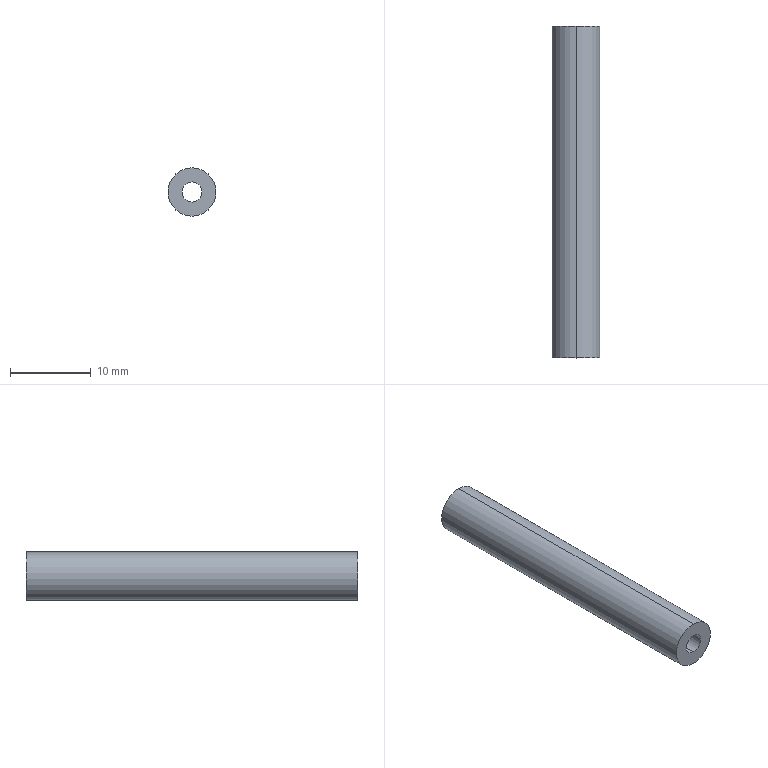Part | SolidWorks | features Extrusion 1, HoleWzd 1 | 1 solid | 6 faces | box 6 x 41.2 x 6 mm | volume 962.663 mm3 | cylinder 4 | plane 2 | commonest cylinder face diameters 2.5 x2 6 x2
STEP:
#1=CARTESIAN_POINT('',(0.,0.,-1.25));
#2=VERTEX_POINT('',#1);
#3=CARTESIAN_POINT('',(0.,0.,1.25));
#4=VERTEX_POINT('',#3);
#5=CARTESIAN_POINT('',(0.,0.,0.));
#6=DIRECTION('',(0.,1.,0.));
#7=DIRECTION('',(0.,0.,1.));
#8=AXIS2_PLACEMENT_3D('',#5,#6,#7);
#9=CIRCLE('',#8,1.25);
#10=EDGE_CURVE('',#2,#4,#9,.T.);
#11=ORIENTED_EDGE('',*,*,#10,.F.);
#12=CARTESIAN_POINT('',(0.,41.2,-1.25));
#13=VERTEX_POINT('',#12);
#14=CARTESIAN_POINT('',(0.,41.2,-1.25));
#15=DIRECTION('',(0.,1.,0.));
#16=VECTOR('',#15,1000.);
#17=LINE('',#14,#16);
#18=EDGE_CURVE('',#2,#13,#17,.T.);
#19=ORIENTED_EDGE('',*,*,#18,.T.);
#20=CARTESIAN_POINT('',(0.,41.2,1.25));
#21=VERTEX_POINT('',#20);
#22=CARTESIAN_POINT('',(0.,41.2,0.));
#23=DIRECTION('',(0.,1.,0.));
#24=DIRECTION('',(0.,0.,1.));
#25=AXIS2_PLACEMENT_3D('',#22,#23,#24);
#26=CIRCLE('',#25,1.25);
#27=EDGE_CURVE('',#13,#21,#26,.T.);
#28=ORIENTED_EDGE('',*,*,#27,.T.);
#29=CARTESIAN_POINT('',(0.,41.2,1.25));
#30=DIRECTION('',(0.,1.,0.));
#31=VECTOR('',#30,1000.);
#32=LINE('',#29,#31);
#33=EDGE_CURVE('',#4,#21,#32,.T.);
#34=ORIENTED_EDGE('',*,*,#33,.F.);
#35=EDGE_LOOP('',(#11,#19,#28,#34));
#36=FACE_OUTER_BOUND('',#35,.T.);
#37=CARTESIAN_POINT('',(0.,41.2,0.));
#38=DIRECTION('',(0.,1.,0.));
#39=DIRECTION('',(0.,0.,1.));
#40=AXIS2_PLACEMENT_3D('',#37,#38,#39);
#41=CYLINDRICAL_SURFACE('',#40,1.25);
#42=ADVANCED_FACE('',(#36),#41,.F.);
#43=CARTESIAN_POINT('',(0.,41.2,3.));
#44=VERTEX_POINT('',#43);
#45=CARTESIAN_POINT('',(0.,41.2,-3.));
#46=VERTEX_POINT('',#45);
#47=CARTESIAN_POINT('',(0.,41.2,0.));
#48=DIRECTION('',(0.,1.,0.));
#49=DIRECTION('',(0.,0.,1.));
#50=AXIS2_PLACEMENT_3D('',#47,#48,#49);
#51=CIRCLE('',#50,3.);
#52=EDGE_CURVE('',#44,#46,#51,.T.);
#53=ORIENTED_EDGE('',*,*,#52,.F.);
#54=CARTESIAN_POINT('',(0.,0.,3.));
#55=VERTEX_POINT('',#54);
#56=CARTESIAN_POINT('',(0.,41.2,3.));
#57=DIRECTION('',(0.,-1.,0.));
#58=VECTOR('',#57,1000.);
#59=LINE('',#56,#58);
#60=EDGE_CURVE('',#44,#55,#59,.T.);
#61=ORIENTED_EDGE('',*,*,#60,.T.);
#62=CARTESIAN_POINT('',(0.,0.,-3.));
#63=VERTEX_POINT('',#62);
#64=CARTESIAN_POINT('',(0.,0.,0.));
#65=DIRECTION('',(0.,1.,0.));
#66=DIRECTION('',(0.,0.,1.));
#67=AXIS2_PLACEMENT_3D('',#64,#65,#66);
#68=CIRCLE('',#67,3.);
#69=EDGE_CURVE('',#55,#63,#68,.T.);
#70=ORIENTED_EDGE('',*,*,#69,.T.);
#71=CARTESIAN_POINT('',(0.,41.2,-3.));
#72=DIRECTION('',(0.,-1.,0.));
#73=VECTOR('',#72,1000.);
#74=LINE('',#71,#73);
#75=EDGE_CURVE('',#46,#63,#74,.T.);
#76=ORIENTED_EDGE('',*,*,#75,.F.);
#77=EDGE_LOOP('',(#53,#61,#70,#76));
#78=FACE_OUTER_BOUND('',#77,.T.);
#79=CARTESIAN_POINT('',(0.,41.2,0.));
#80=DIRECTION('',(0.,-1.,0.));
#81=DIRECTION('',(0.,0.,-1.));
#82=AXIS2_PLACEMENT_3D('',#79,#80,#81);
#83=CYLINDRICAL_SURFACE('',#82,3.);
#84=ADVANCED_FACE('',(#78),#83,.T.);
#85=ORIENTED_EDGE('',*,*,#60,.F.);
#86=CARTESIAN_POINT('',(0.,41.2,0.));
#87=DIRECTION('',(0.,1.,0.));
#88=DIRECTION('',(0.,0.,1.));
#89=AXIS2_PLACEMENT_3D('',#86,#87,#88);
#90=CIRCLE('',#89,3.);
#91=EDGE_CURVE('',#46,#44,#90,.T.);
#92=ORIENTED_EDGE('',*,*,#91,.F.);
#93=ORIENTED_EDGE('',*,*,#75,.T.);
#94=CARTESIAN_POINT('',(0.,0.,0.));
#95=DIRECTION('',(0.,1.,0.));
#96=DIRECTION('',(0.,0.,1.));
#97=AXIS2_PLACEMENT_3D('',#94,#95,#96);
#98=CIRCLE('',#97,3.);
#99=EDGE_CURVE('',#63,#55,#98,.T.);
#100=ORIENTED_EDGE('',*,*,#99,.T.);
#101=EDGE_LOOP('',(#85,#92,#93,#100));
#102=FACE_OUTER_BOUND('',#101,.T.);
#103=CARTESIAN_POINT('',(0.,41.2,0.));
#104=DIRECTION('',(0.,-1.,0.));
#105=DIRECTION('',(0.,0.,-1.));
#106=AXIS2_PLACEMENT_3D('',#103,#104,#105);
#107=CYLINDRICAL_SURFACE('',#106,3.);
#108=ADVANCED_FACE('',(#102),#107,.T.);
#109=CARTESIAN_POINT('',(0.,41.2,0.));
#110=DIRECTION('',(0.,1.,0.));
#111=DIRECTION('',(0.,0.,1.));
#112=AXIS2_PLACEMENT_3D('',#109,#110,#111);
#113=CIRCLE('',#112,1.25);
#114=EDGE_CURVE('',#21,#13,#113,.T.);
#115=ORIENTED_EDGE('',*,*,#114,.F.);
#116=ORIENTED_EDGE('',*,*,#27,.F.);
#117=EDGE_LOOP('',(#115,#116));
#118=FACE_BOUND('',#117,.T.);
#119=ORIENTED_EDGE('',*,*,#91,.T.);
#120=ORIENTED_EDGE('',*,*,#52,.T.);
#121=EDGE_LOOP('',(#119,#120));
#122=FACE_OUTER_BOUND('',#121,.T.);
#123=CARTESIAN_POINT('',(0.,41.2,0.));
#124=DIRECTION('',(0.,1.,0.));
#125=DIRECTION('',(0.,0.,1.));
#126=AXIS2_PLACEMENT_3D('',#123,#124,#125);
#127=PLANE('',#126);
#128=ADVANCED_FACE('',(#118,#122),#127,.T.);
#129=CARTESIAN_POINT('',(0.,0.,0.));
#130=DIRECTION('',(0.,1.,0.));
#131=DIRECTION('',(0.,0.,1.));
#132=AXIS2_PLACEMENT_3D('',#129,#130,#131);
#133=CIRCLE('',#132,1.25);
#134=EDGE_CURVE('',#4,#2,#133,.T.);
#135=ORIENTED_EDGE('',*,*,#134,.T.);
#136=ORIENTED_EDGE('',*,*,#10,.T.);
#137=EDGE_LOOP('',(#135,#136));
#138=FACE_BOUND('',#137,.T.);
#139=ORIENTED_EDGE('',*,*,#99,.F.);
#140=ORIENTED_EDGE('',*,*,#69,.F.);
#141=EDGE_LOOP('',(#139,#140));
#142=FACE_OUTER_BOUND('',#141,.T.);
#143=CARTESIAN_POINT('',(0.,0.,0.));
#144=DIRECTION('',(0.,1.,0.));
#145=DIRECTION('',(0.,0.,1.));
#146=AXIS2_PLACEMENT_3D('',#143,#144,#145);
#147=PLANE('',#146);
#148=ADVANCED_FACE('',(#138,#142),#147,.F.);
#149=ORIENTED_EDGE('',*,*,#18,.F.);
#150=ORIENTED_EDGE('',*,*,#134,.F.);
#151=ORIENTED_EDGE('',*,*,#33,.T.);
#152=ORIENTED_EDGE('',*,*,#114,.T.);
#153=EDGE_LOOP('',(#149,#150,#151,#152));
#154=FACE_OUTER_BOUND('',#153,.T.);
#155=CARTESIAN_POINT('',(0.,41.2,0.));
#156=DIRECTION('',(0.,1.,0.));
#157=DIRECTION('',(0.,0.,1.));
#158=AXIS2_PLACEMENT_3D('',#155,#156,#157);
#159=CYLINDRICAL_SURFACE('',#158,1.25);
#160=ADVANCED_FACE('',(#154),#159,.F.);
#161=CLOSED_SHELL('',(#42,#84,#108,#128,#148,#160));
#162=MANIFOLD_SOLID_BREP('',#161);
#163=CARTESIAN_POINT('',(0.,0.,0.));
#164=DIRECTION('',(0.,0.,1.));
#165=DIRECTION('',(1.,0.,0.));
#166=AXIS2_PLACEMENT_3D('',#163,#164,#165);
#167=(LENGTH_UNIT()NAMED_UNIT(*)SI_UNIT(.MILLI.,.METRE.));
#168=UNCERTAINTY_MEASURE_WITH_UNIT(LENGTH_MEASURE(0.00001),#167,'','');
#169=(NAMED_UNIT(*)PLANE_ANGLE_UNIT()SI_UNIT($,.RADIAN.));
#170=(NAMED_UNIT(*)SI_UNIT($,.STERADIAN.)SOLID_ANGLE_UNIT());
#171=(GEOMETRIC_REPRESENTATION_CONTEXT(3)GLOBAL_UNCERTAINTY_ASSIGNED_CONTEXT((#168))GLOBAL_UNIT_ASSIGNED_CONTEXT((#167,#169,#170))REPRESENTATION_CONTEXT('',''));
#172=ADVANCED_BREP_SHAPE_REPRESENTATION('',(#162,#166),#171);